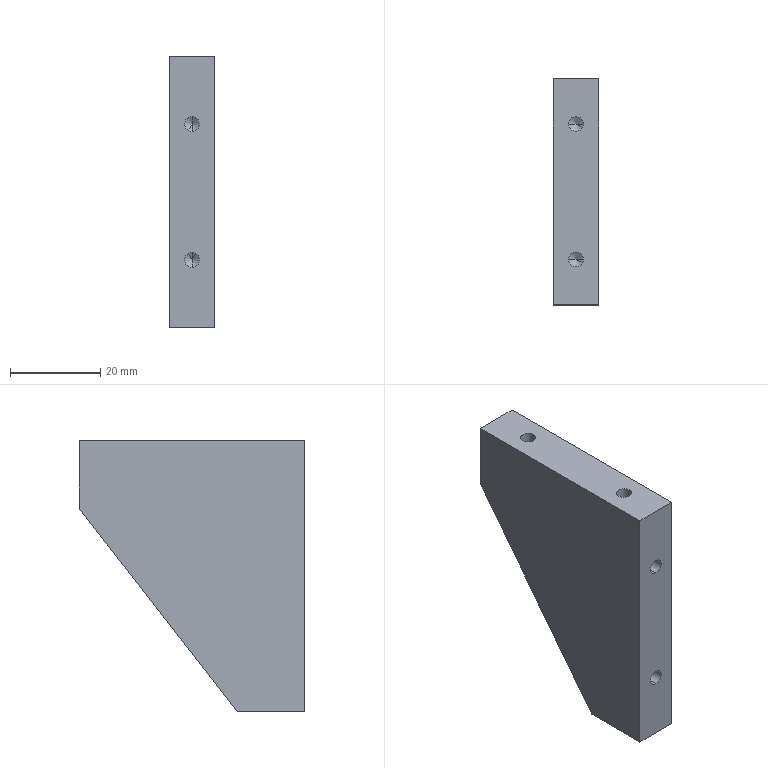Part | STEP file | 03-22 Lead screw fixing plate rib | 1 solid | 23 faces | box 10 x 50 x 60 mm | volume 21700 mm3 | cylinder 8 | cone 8 | plane 7 | commonest cylinder face diameters 3.3 x8